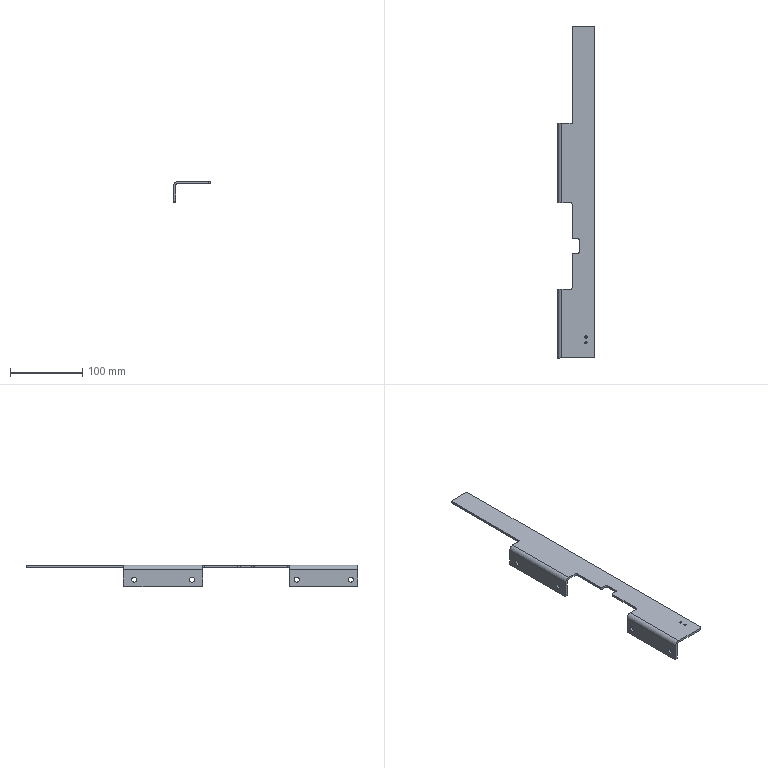Part | NX | features 5003_221_Bracket 2 | 1 solid | 43 faces | box 51 x 460 x 30 mm | volume 69398 mm3 | cylinder 21 | plane 20 | cone 2 | commonest cylinder face diameters 4 x11 7 x4 2.5 x2 6 x2 12 x2
STEP:
#1=CARTESIAN_POINT('',(224.525,-262.,-58.));
#2=VERTEX_POINT('',#1);
#3=CARTESIAN_POINT('',(224.525,-152.,-58.));
#4=VERTEX_POINT('',#3);
#5=CARTESIAN_POINT('',(224.525,-477.,-58.));
#6=DIRECTION('',(0.,1.,0.));
#7=VECTOR('',#6,1000.);
#8=LINE('',#5,#7);
#9=EDGE_CURVE('',#2,#4,#8,.T.);
#10=ORIENTED_EDGE('',*,*,#9,.T.);
#11=CARTESIAN_POINT('',(218.525,-152.,-64.));
#12=VERTEX_POINT('',#11);
#13=CARTESIAN_POINT('',(224.525,-152.,-64.));
#14=DIRECTION('',(0.,-1.,0.));
#15=DIRECTION('',(1.,0.,0.));
#16=AXIS2_PLACEMENT_3D('',#13,#14,#15);
#17=CIRCLE('',#16,6.);
#18=EDGE_CURVE('',#12,#4,#17,.F.);
#19=ORIENTED_EDGE('',*,*,#18,.F.);
#20=CARTESIAN_POINT('',(218.525,-262.,-64.));
#21=VERTEX_POINT('',#20);
#22=CARTESIAN_POINT('',(218.525,-477.,-64.));
#23=DIRECTION('',(0.,1.,0.));
#24=VECTOR('',#23,1000.);
#25=LINE('',#22,#24);
#26=EDGE_CURVE('',#21,#12,#25,.T.);
#27=ORIENTED_EDGE('',*,*,#26,.F.);
#28=CARTESIAN_POINT('',(224.525,-262.,-64.));
#29=DIRECTION('',(0.,1.,0.));
#30=DIRECTION('',(-1.,0.,0.));
#31=AXIS2_PLACEMENT_3D('',#28,#29,#30);
#32=CIRCLE('',#31,6.);
#33=EDGE_CURVE('',#2,#21,#32,.F.);
#34=ORIENTED_EDGE('',*,*,#33,.F.);
#35=EDGE_LOOP('',(#10,#19,#27,#34));
#36=FACE_BOUND('',#35,.T.);
#37=CARTESIAN_POINT('',(224.525,-477.,-64.));
#38=DIRECTION('',(0.,1.,0.));
#39=DIRECTION('',(-1.,0.,0.));
#40=AXIS2_PLACEMENT_3D('',#37,#38,#39);
#41=CYLINDRICAL_SURFACE('',#40,6.);
#42=ADVANCED_FACE('',(#36),#41,.T.);
#43=CARTESIAN_POINT('',(218.525,-167.,-74.5));
#44=VERTEX_POINT('',#43);
#45=CARTESIAN_POINT('',(218.525,-167.,-78.));
#46=DIRECTION('',(1.,0.,0.));
#47=DIRECTION('',(0.,0.,1.));
#48=AXIS2_PLACEMENT_3D('',#45,#46,#47);
#49=CIRCLE('',#48,3.5);
#50=EDGE_CURVE('',#44,#44,#49,.T.);
#51=ORIENTED_EDGE('',*,*,#50,.T.);
#52=EDGE_LOOP('',(#51));
#53=FACE_BOUND('',#52,.T.);
#54=CARTESIAN_POINT('',(218.525,-247.,-74.5));
#55=VERTEX_POINT('',#54);
#56=CARTESIAN_POINT('',(218.525,-247.,-78.));
#57=DIRECTION('',(1.,0.,0.));
#58=DIRECTION('',(0.,0.,1.));
#59=AXIS2_PLACEMENT_3D('',#56,#57,#58);
#60=CIRCLE('',#59,3.5);
#61=EDGE_CURVE('',#55,#55,#60,.T.);
#62=ORIENTED_EDGE('',*,*,#61,.T.);
#63=EDGE_LOOP('',(#62));
#64=FACE_BOUND('',#63,.T.);
#65=CARTESIAN_POINT('',(218.525,-152.,-86.));
#66=VERTEX_POINT('',#65);
#67=CARTESIAN_POINT('',(218.525,-152.,-57.999));
#68=DIRECTION('',(0.,0.,-1.));
#69=VECTOR('',#68,1000.);
#70=LINE('',#67,#69);
#71=EDGE_CURVE('',#12,#66,#70,.T.);
#72=ORIENTED_EDGE('',*,*,#71,.T.);
#73=CARTESIAN_POINT('',(218.525,-154.,-88.));
#74=VERTEX_POINT('',#73);
#75=CARTESIAN_POINT('',(218.525,-154.,-86.));
#76=DIRECTION('',(1.,0.,0.));
#77=DIRECTION('',(0.,0.,1.));
#78=AXIS2_PLACEMENT_3D('',#75,#76,#77);
#79=CIRCLE('',#78,2.);
#80=EDGE_CURVE('',#66,#74,#79,.F.);
#81=ORIENTED_EDGE('',*,*,#80,.T.);
#82=CARTESIAN_POINT('',(218.525,-260.,-88.));
#83=VERTEX_POINT('',#82);
#84=CARTESIAN_POINT('',(218.525,-477.,-88.));
#85=DIRECTION('',(0.,1.,0.));
#86=VECTOR('',#85,1000.);
#87=LINE('',#84,#86);
#88=EDGE_CURVE('',#83,#74,#87,.T.);
#89=ORIENTED_EDGE('',*,*,#88,.F.);
#90=CARTESIAN_POINT('',(218.525,-262.,-86.));
#91=VERTEX_POINT('',#90);
#92=CARTESIAN_POINT('',(218.525,-260.,-86.));
#93=DIRECTION('',(1.,0.,0.));
#94=DIRECTION('',(0.,0.,1.));
#95=AXIS2_PLACEMENT_3D('',#92,#93,#94);
#96=CIRCLE('',#95,2.);
#97=EDGE_CURVE('',#83,#91,#96,.F.);
#98=ORIENTED_EDGE('',*,*,#97,.T.);
#99=CARTESIAN_POINT('',(218.525,-262.,-57.999));
#100=DIRECTION('',(0.,0.,-1.));
#101=VECTOR('',#100,1000.);
#102=LINE('',#99,#101);
#103=EDGE_CURVE('',#21,#91,#102,.T.);
#104=ORIENTED_EDGE('',*,*,#103,.F.);
#105=ORIENTED_EDGE('',*,*,#26,.T.);
#106=EDGE_LOOP('',(#72,#81,#89,#98,#104,#105));
#107=FACE_BOUND('',#106,.T.);
#108=CARTESIAN_POINT('',(218.525,-477.,-64.));
#109=DIRECTION('',(1.,0.,0.));
#110=DIRECTION('',(0.,0.,1.));
#111=AXIS2_PLACEMENT_3D('',#108,#109,#110);
#112=PLANE('',#111);
#113=ADVANCED_FACE('',(#53,#64,#107),#112,.F.);
#114=ORIENTED_EDGE('',*,*,#88,.T.);
#115=CARTESIAN_POINT('',(221.525,-154.,-88.));
#116=VERTEX_POINT('',#115);
#117=CARTESIAN_POINT('',(218.525,-154.,-88.));
#118=DIRECTION('',(-1.,0.,0.));
#119=VECTOR('',#118,1000.);
#120=LINE('',#117,#119);
#121=EDGE_CURVE('',#74,#116,#120,.F.);
#122=ORIENTED_EDGE('',*,*,#121,.T.);
#123=CARTESIAN_POINT('',(221.525,-260.,-88.));
#124=VERTEX_POINT('',#123);
#125=CARTESIAN_POINT('',(221.525,-477.,-88.));
#126=DIRECTION('',(0.,1.,0.));
#127=VECTOR('',#126,1000.);
#128=LINE('',#125,#127);
#129=EDGE_CURVE('',#124,#116,#128,.T.);
#130=ORIENTED_EDGE('',*,*,#129,.F.);
#131=CARTESIAN_POINT('',(218.525,-260.,-88.));
#132=DIRECTION('',(1.,0.,0.));
#133=VECTOR('',#132,1000.);
#134=LINE('',#131,#133);
#135=EDGE_CURVE('',#124,#83,#134,.F.);
#136=ORIENTED_EDGE('',*,*,#135,.T.);
#137=EDGE_LOOP('',(#114,#122,#130,#136));
#138=FACE_BOUND('',#137,.T.);
#139=CARTESIAN_POINT('',(218.525,-477.,-88.));
#140=DIRECTION('',(0.,0.,1.));
#141=DIRECTION('',(0.,-1.,0.));
#142=AXIS2_PLACEMENT_3D('',#139,#140,#141);
#143=PLANE('',#142);
#144=ADVANCED_FACE('',(#138),#143,.F.);
#145=CARTESIAN_POINT('',(221.525,-167.,-74.5));
#146=VERTEX_POINT('',#145);
#147=CARTESIAN_POINT('',(221.525,-167.,-78.));
#148=DIRECTION('',(1.,0.,0.));
#149=DIRECTION('',(0.,0.,1.));
#150=AXIS2_PLACEMENT_3D('',#147,#148,#149);
#151=CIRCLE('',#150,3.5);
#152=EDGE_CURVE('',#146,#146,#151,.T.);
#153=ORIENTED_EDGE('',*,*,#152,.F.);
#154=EDGE_LOOP('',(#153));
#155=FACE_BOUND('',#154,.T.);
#156=CARTESIAN_POINT('',(221.525,-247.,-74.5));
#157=VERTEX_POINT('',#156);
#158=CARTESIAN_POINT('',(221.525,-247.,-78.));
#159=DIRECTION('',(1.,0.,0.));
#160=DIRECTION('',(0.,0.,1.));
#161=AXIS2_PLACEMENT_3D('',#158,#159,#160);
#162=CIRCLE('',#161,3.5);
#163=EDGE_CURVE('',#157,#157,#162,.T.);
#164=ORIENTED_EDGE('',*,*,#163,.F.);
#165=EDGE_LOOP('',(#164));
#166=FACE_BOUND('',#165,.T.);
#167=ORIENTED_EDGE('',*,*,#129,.T.);
#168=CARTESIAN_POINT('',(221.525,-152.,-86.));
#169=VERTEX_POINT('',#168);
#170=CARTESIAN_POINT('',(221.525,-154.,-86.));
#171=DIRECTION('',(-1.,0.,0.));
#172=DIRECTION('',(0.,0.,-1.));
#173=AXIS2_PLACEMENT_3D('',#170,#171,#172);
#174=CIRCLE('',#173,2.);
#175=EDGE_CURVE('',#116,#169,#174,.F.);
#176=ORIENTED_EDGE('',*,*,#175,.T.);
#177=CARTESIAN_POINT('',(221.525,-152.,-64.));
#178=VERTEX_POINT('',#177);
#179=CARTESIAN_POINT('',(221.525,-152.,-57.999));
#180=DIRECTION('',(0.,0.,-1.));
#181=VECTOR('',#180,1000.);
#182=LINE('',#179,#181);
#183=EDGE_CURVE('',#178,#169,#182,.T.);
#184=ORIENTED_EDGE('',*,*,#183,.F.);
#185=CARTESIAN_POINT('',(221.525,-262.,-64.));
#186=VERTEX_POINT('',#185);
#187=CARTESIAN_POINT('',(221.525,-477.,-64.));
#188=DIRECTION('',(0.,1.,0.));
#189=VECTOR('',#188,1000.);
#190=LINE('',#187,#189);
#191=EDGE_CURVE('',#186,#178,#190,.T.);
#192=ORIENTED_EDGE('',*,*,#191,.F.);
#193=CARTESIAN_POINT('',(221.525,-262.,-86.));
#194=VERTEX_POINT('',#193);
#195=CARTESIAN_POINT('',(221.525,-262.,-57.999));
#196=DIRECTION('',(0.,0.,1.));
#197=VECTOR('',#196,1000.);
#198=LINE('',#195,#197);
#199=EDGE_CURVE('',#194,#186,#198,.T.);
#200=ORIENTED_EDGE('',*,*,#199,.F.);
#201=CARTESIAN_POINT('',(221.525,-260.,-86.));
#202=DIRECTION('',(-1.,0.,0.));
#203=DIRECTION('',(0.,0.,-1.));
#204=AXIS2_PLACEMENT_3D('',#201,#202,#203);
#205=CIRCLE('',#204,2.);
#206=EDGE_CURVE('',#194,#124,#205,.F.);
#207=ORIENTED_EDGE('',*,*,#206,.T.);
#208=EDGE_LOOP('',(#167,#176,#184,#192,#200,#207));
#209=FACE_BOUND('',#208,.T.);
#210=CARTESIAN_POINT('',(221.525,-477.,-88.));
#211=DIRECTION('',(-1.,0.,0.));
#212=DIRECTION('',(0.,0.,-1.));
#213=AXIS2_PLACEMENT_3D('',#210,#211,#212);
#214=PLANE('',#213);
#215=ADVANCED_FACE('',(#155,#166,#209),#214,.F.);
#216=ORIENTED_EDGE('',*,*,#191,.T.);
#217=CARTESIAN_POINT('',(224.525,-152.,-61.));
#218=VERTEX_POINT('',#217);
#219=CARTESIAN_POINT('',(224.525,-152.,-64.));
#220=DIRECTION('',(0.,-1.,0.));
#221=DIRECTION('',(1.,0.,0.));
#222=AXIS2_PLACEMENT_3D('',#219,#220,#221);
#223=CIRCLE('',#222,3.);
#224=EDGE_CURVE('',#218,#178,#223,.T.);
#225=ORIENTED_EDGE('',*,*,#224,.F.);
#226=CARTESIAN_POINT('',(224.525,-262.,-61.));
#227=VERTEX_POINT('',#226);
#228=CARTESIAN_POINT('',(224.525,-477.,-61.));
#229=DIRECTION('',(0.,1.,0.));
#230=VECTOR('',#229,1000.);
#231=LINE('',#228,#230);
#232=EDGE_CURVE('',#227,#218,#231,.T.);
#233=ORIENTED_EDGE('',*,*,#232,.F.);
#234=CARTESIAN_POINT('',(224.525,-262.,-64.));
#235=DIRECTION('',(0.,1.,0.));
#236=DIRECTION('',(-1.,0.,0.));
#237=AXIS2_PLACEMENT_3D('',#234,#235,#236);
#238=CIRCLE('',#237,3.);
#239=EDGE_CURVE('',#186,#227,#238,.T.);
#240=ORIENTED_EDGE('',*,*,#239,.F.);
#241=EDGE_LOOP('',(#216,#225,#233,#240));
#242=FACE_BOUND('',#241,.T.);
#243=CARTESIAN_POINT('',(224.525,-477.,-64.));
#244=DIRECTION('',(0.,1.,0.));
#245=DIRECTION('',(-1.,0.,0.));
#246=AXIS2_PLACEMENT_3D('',#243,#244,#245);
#247=CYLINDRICAL_SURFACE('',#246,3.);
#248=ADVANCED_FACE('',(#242),#247,.F.);
#249=CARTESIAN_POINT('',(269.525,-475.,-61.));
#250=VERTEX_POINT('',#249);
#251=CARTESIAN_POINT('',(269.525,-19.,-61.));
#252=VERTEX_POINT('',#251);
#253=CARTESIAN_POINT('',(269.525,-477.,-61.));
#254=DIRECTION('',(0.,1.,0.));
#255=VECTOR('',#254,1000.);
#256=LINE('',#253,#255);
#257=EDGE_CURVE('',#250,#252,#256,.T.);
#258=ORIENTED_EDGE('',*,*,#257,.T.);
#259=CARTESIAN_POINT('',(269.525,-19.,-58.));
#260=VERTEX_POINT('',#259);
#261=CARTESIAN_POINT('',(269.525,-19.,-58.));
#262=DIRECTION('',(0.,0.,1.));
#263=VECTOR('',#262,1000.);
#264=LINE('',#261,#263);
#265=EDGE_CURVE('',#252,#260,#264,.T.);
#266=ORIENTED_EDGE('',*,*,#265,.T.);
#267=CARTESIAN_POINT('',(269.525,-475.,-58.));
#268=VERTEX_POINT('',#267);
#269=CARTESIAN_POINT('',(269.525,-477.,-58.));
#270=DIRECTION('',(0.,1.,0.));
#271=VECTOR('',#270,1000.);
#272=LINE('',#269,#271);
#273=EDGE_CURVE('',#268,#260,#272,.T.);
#274=ORIENTED_EDGE('',*,*,#273,.F.);
#275=CARTESIAN_POINT('',(269.525,-475.,-58.));
#276=DIRECTION('',(0.,0.,1.));
#277=VECTOR('',#276,1000.);
#278=LINE('',#275,#277);
#279=EDGE_CURVE('',#268,#250,#278,.F.);
#280=ORIENTED_EDGE('',*,*,#279,.T.);
#281=EDGE_LOOP('',(#258,#266,#274,#280));
#282=FACE_BOUND('',#281,.T.);
#283=CARTESIAN_POINT('',(269.525,-477.,-58.));
#284=DIRECTION('',(-1.,0.,0.));
#285=DIRECTION('',(0.,-1.,0.));
#286=AXIS2_PLACEMENT_3D('',#283,#284,#285);
#287=PLANE('',#286);
#288=ADVANCED_FACE('',(#282),#287,.F.);
#289=CARTESIAN_POINT('',(257.825,-457.565,-58.));
#290=VERTEX_POINT('',#289);
#291=CARTESIAN_POINT('',(257.825,-456.04,-58.));
#292=DIRECTION('',(0.,0.,1.));
#293=DIRECTION('',(0.,-1.,0.));
#294=AXIS2_PLACEMENT_3D('',#291,#292,#293);
#295=CIRCLE('',#294,1.525);
#296=EDGE_CURVE('',#290,#290,#295,.T.);
#297=ORIENTED_EDGE('',*,*,#296,.F.);
#298=EDGE_LOOP('',(#297));
#299=FACE_BOUND('',#298,.T.);
#300=CARTESIAN_POINT('',(257.825,-449.565,-58.));
#301=VERTEX_POINT('',#300);
#302=CARTESIAN_POINT('',(257.825,-448.04,-58.));
#303=DIRECTION('',(0.,0.,1.));
#304=DIRECTION('',(0.,-1.,0.));
#305=AXIS2_PLACEMENT_3D('',#302,#303,#304);
#306=CIRCLE('',#305,1.525);
#307=EDGE_CURVE('',#301,#301,#306,.T.);
#308=ORIENTED_EDGE('',*,*,#307,.F.);
#309=EDGE_LOOP('',(#308));
#310=FACE_BOUND('',#309,.T.);
#311=CARTESIAN_POINT('',(238.525,-310.,-58.));
#312=VERTEX_POINT('',#311);
#313=CARTESIAN_POINT('',(238.525,-264.,-58.));
#314=VERTEX_POINT('',#313);
#315=CARTESIAN_POINT('',(238.525,-312.,-58.));
#316=DIRECTION('',(0.,1.,0.));
#317=VECTOR('',#316,1000.);
#318=LINE('',#315,#317);
#319=EDGE_CURVE('',#312,#314,#318,.T.);
#320=ORIENTED_EDGE('',*,*,#319,.F.);
#321=CARTESIAN_POINT('',(240.525,-312.,-58.));
#322=VERTEX_POINT('',#321);
#323=CARTESIAN_POINT('',(240.525,-310.,-58.));
#324=DIRECTION('',(0.,0.,-1.));
#325=DIRECTION('',(0.,1.,0.));
#326=AXIS2_PLACEMENT_3D('',#323,#324,#325);
#327=CIRCLE('',#326,2.);
#328=EDGE_CURVE('',#312,#322,#327,.F.);
#329=ORIENTED_EDGE('',*,*,#328,.T.);
#330=CARTESIAN_POINT('',(246.525,-312.,-58.));
#331=VERTEX_POINT('',#330);
#332=CARTESIAN_POINT('',(248.525,-312.,-58.));
#333=DIRECTION('',(-1.,0.,0.));
#334=VECTOR('',#333,1000.);
#335=LINE('',#332,#334);
#336=EDGE_CURVE('',#331,#322,#335,.T.);
#337=ORIENTED_EDGE('',*,*,#336,.F.);
#338=CARTESIAN_POINT('',(248.525,-314.,-58.));
#339=VERTEX_POINT('',#338);
#340=CARTESIAN_POINT('',(246.525,-314.,-58.));
#341=DIRECTION('',(0.,0.,-1.));
#342=DIRECTION('',(0.,1.,0.));
#343=AXIS2_PLACEMENT_3D('',#340,#341,#342);
#344=CIRCLE('',#343,2.);
#345=EDGE_CURVE('',#331,#339,#344,.T.);
#346=ORIENTED_EDGE('',*,*,#345,.T.);
#347=CARTESIAN_POINT('',(248.525,-330.,-58.));
#348=VERTEX_POINT('',#347);
#349=CARTESIAN_POINT('',(248.525,-332.,-58.));
#350=DIRECTION('',(0.,1.,0.));
#351=VECTOR('',#350,1000.);
#352=LINE('',#349,#351);
#353=EDGE_CURVE('',#348,#339,#352,.T.);
#354=ORIENTED_EDGE('',*,*,#353,.F.);
#355=CARTESIAN_POINT('',(246.525,-332.,-58.));
#356=VERTEX_POINT('',#355);
#357=CARTESIAN_POINT('',(246.525,-330.,-58.));
#358=DIRECTION('',(0.,0.,-1.));
#359=DIRECTION('',(0.,1.,0.));
#360=AXIS2_PLACEMENT_3D('',#357,#358,#359);
#361=CIRCLE('',#360,2.);
#362=EDGE_CURVE('',#348,#356,#361,.T.);
#363=ORIENTED_EDGE('',*,*,#362,.T.);
#364=CARTESIAN_POINT('',(240.525,-332.,-58.));
#365=VERTEX_POINT('',#364);
#366=CARTESIAN_POINT('',(238.525,-332.,-58.));
#367=DIRECTION('',(1.,0.,0.));
#368=VECTOR('',#367,1000.);
#369=LINE('',#366,#368);
#370=EDGE_CURVE('',#365,#356,#369,.T.);
#371=ORIENTED_EDGE('',*,*,#370,.F.);
#372=CARTESIAN_POINT('',(238.525,-334.,-58.));
#373=VERTEX_POINT('',#372);
#374=CARTESIAN_POINT('',(240.525,-334.,-58.));
#375=DIRECTION('',(0.,0.,-1.));
#376=DIRECTION('',(0.,1.,0.));
#377=AXIS2_PLACEMENT_3D('',#374,#375,#376);
#378=CIRCLE('',#377,2.);
#379=EDGE_CURVE('',#365,#373,#378,.F.);
#380=ORIENTED_EDGE('',*,*,#379,.T.);
#381=CARTESIAN_POINT('',(238.525,-380.,-58.));
#382=VERTEX_POINT('',#381);
#383=CARTESIAN_POINT('',(238.525,-382.,-58.));
#384=DIRECTION('',(0.,1.,0.));
#385=VECTOR('',#384,1000.);
#386=LINE('',#383,#385);
#387=EDGE_CURVE('',#382,#373,#386,.T.);
#388=ORIENTED_EDGE('',*,*,#387,.F.);
#389=CARTESIAN_POINT('',(236.525,-382.,-58.));
#390=VERTEX_POINT('',#389);
#391=CARTESIAN_POINT('',(236.525,-380.,-58.));
#392=DIRECTION('',(0.,0.,-1.));
#393=DIRECTION('',(0.,1.,0.));
#394=AXIS2_PLACEMENT_3D('',#391,#392,#393);
#395=CIRCLE('',#394,2.);
#396=EDGE_CURVE('',#382,#390,#395,.T.);
#397=ORIENTED_EDGE('',*,*,#396,.T.);
#398=CARTESIAN_POINT('',(224.525,-382.,-58.));
#399=VERTEX_POINT('',#398);
#400=CARTESIAN_POINT('',(238.525,-382.,-58.));
#401=DIRECTION('',(1.,0.,0.));
#402=VECTOR('',#401,1000.);
#403=LINE('',#400,#402);
#404=EDGE_CURVE('',#399,#390,#403,.T.);
#405=ORIENTED_EDGE('',*,*,#404,.F.);
#406=CARTESIAN_POINT('',(224.525,-477.,-58.));
#407=VERTEX_POINT('',#406);
#408=CARTESIAN_POINT('',(224.525,-477.,-58.));
#409=DIRECTION('',(0.,1.,0.));
#410=VECTOR('',#409,1000.);
#411=LINE('',#408,#410);
#412=EDGE_CURVE('',#407,#399,#411,.T.);
#413=ORIENTED_EDGE('',*,*,#412,.F.);
#414=CARTESIAN_POINT('',(267.525,-477.,-58.));
#415=VERTEX_POINT('',#414);
#416=CARTESIAN_POINT('',(224.525,-477.,-58.));
#417=DIRECTION('',(-1.,0.,0.));
#418=VECTOR('',#417,1000.);
#419=LINE('',#416,#418);
#420=EDGE_CURVE('',#415,#407,#419,.T.);
#421=ORIENTED_EDGE('',*,*,#420,.F.);
#422=CARTESIAN_POINT('',(267.525,-475.,-58.));
#423=DIRECTION('',(0.,0.,-1.));
#424=DIRECTION('',(0.,1.,0.));
#425=AXIS2_PLACEMENT_3D('',#422,#423,#424);
#426=CIRCLE('',#425,2.);
#427=EDGE_CURVE('',#415,#268,#426,.F.);
#428=ORIENTED_EDGE('',*,*,#427,.T.);
#429=ORIENTED_EDGE('',*,*,#273,.T.);
#430=CARTESIAN_POINT('',(267.525,-17.,-58.));
#431=VERTEX_POINT('',#430);
#432=CARTESIAN_POINT('',(267.525,-19.,-58.));
#433=DIRECTION('',(0.,0.,-1.));
#434=DIRECTION('',(0.,1.,0.));
#435=AXIS2_PLACEMENT_3D('',#432,#433,#434);
#436=CIRCLE('',#435,2.);
#437=EDGE_CURVE('',#260,#431,#436,.F.);
#438=ORIENTED_EDGE('',*,*,#437,.T.);
#439=CARTESIAN_POINT('',(238.525,-17.,-58.));
#440=VERTEX_POINT('',#439);
#441=CARTESIAN_POINT('',(224.525,-17.,-58.));
#442=DIRECTION('',(-1.,0.,0.));
#443=VECTOR('',#442,1000.);
#444=LINE('',#441,#443);
#445=EDGE_CURVE('',#431,#440,#444,.T.);
#446=ORIENTED_EDGE('',*,*,#445,.T.);
#447=CARTESIAN_POINT('',(238.525,-152.,-58.));
#448=VERTEX_POINT('',#447);
#449=CARTESIAN_POINT('',(238.525,-152.,-58.));
#450=DIRECTION('',(0.,1.,0.));
#451=VECTOR('',#450,1000.);
#452=LINE('',#449,#451);
#453=EDGE_CURVE('',#448,#440,#452,.T.);
#454=ORIENTED_EDGE('',*,*,#453,.F.);
#455=CARTESIAN_POINT('',(218.525,-152.,-58.));
#456=DIRECTION('',(1.,0.,0.));
#457=VECTOR('',#456,1000.);
#458=LINE('',#455,#457);
#459=EDGE_CURVE('',#4,#448,#458,.T.);
#460=ORIENTED_EDGE('',*,*,#459,.F.);
#461=ORIENTED_EDGE('',*,*,#9,.F.);
#462=CARTESIAN_POINT('',(236.525,-262.,-58.));
#463=VERTEX_POINT('',#462);
#464=CARTESIAN_POINT('',(238.525,-262.,-58.));
#465=DIRECTION('',(-1.,0.,0.));
#466=VECTOR('',#465,1000.);
#467=LINE('',#464,#466);
#468=EDGE_CURVE('',#463,#2,#467,.T.);
#469=ORIENTED_EDGE('',*,*,#468,.F.);
#470=CARTESIAN_POINT('',(236.525,-264.,-58.));
#471=DIRECTION('',(0.,0.,-1.));
#472=DIRECTION('',(0.,1.,0.));
#473=AXIS2_PLACEMENT_3D('',#470,#471,#472);
#474=CIRCLE('',#473,2.);
#475=EDGE_CURVE('',#463,#314,#474,.T.);
#476=ORIENTED_EDGE('',*,*,#475,.T.);
#477=EDGE_LOOP('',(#320,#329,#337,#346,#354,#363,#371,#380,#388,#397,#405,#413,#421,#428,#429,#438,#446,#454,#460,#461,#469,#476));
#478=FACE_BOUND('',#477,.T.);
#479=CARTESIAN_POINT('',(224.525,-477.,-58.));
#480=DIRECTION('',(0.,0.,-1.));
#481=DIRECTION('',(0.,1.,0.));
#482=AXIS2_PLACEMENT_3D('',#479,#480,#481);
#483=PLANE('',#482);
#484=ADVANCED_FACE('',(#299,#310,#478),#483,.F.);
#485=ORIENTED_EDGE('',*,*,#412,.T.);
#486=CARTESIAN_POINT('',(218.525,-382.,-64.));
#487=VERTEX_POINT('',#486);
#488=CARTESIAN_POINT('',(224.525,-382.,-64.));
#489=DIRECTION('',(0.,-1.,0.));
#490=DIRECTION('',(1.,0.,0.));
#491=AXIS2_PLACEMENT_3D('',#488,#489,#490);
#492=CIRCLE('',#491,6.);
#493=EDGE_CURVE('',#487,#399,#492,.F.);
#494=ORIENTED_EDGE('',*,*,#493,.F.);
#495=CARTESIAN_POINT('',(218.525,-477.,-64.));
#496=VERTEX_POINT('',#495);
#497=CARTESIAN_POINT('',(218.525,-477.,-64.));
#498=DIRECTION('',(0.,1.,0.));
#499=VECTOR('',#498,1000.);
#500=LINE('',#497,#499);
#501=EDGE_CURVE('',#496,#487,#500,.T.);
#502=ORIENTED_EDGE('',*,*,#501,.F.);
#503=CARTESIAN_POINT('',(224.525,-477.,-64.));
#504=DIRECTION('',(0.,-1.,0.));
#505=DIRECTION('',(-1.,0.,0.));
#506=AXIS2_PLACEMENT_3D('',#503,#504,#505);
#507=CIRCLE('',#506,6.);
#508=EDGE_CURVE('',#407,#496,#507,.T.);
#509=ORIENTED_EDGE('',*,*,#508,.F.);
#510=EDGE_LOOP('',(#485,#494,#502,#509));
#511=FACE_BOUND('',#510,.T.);
#512=CARTESIAN_POINT('',(224.525,-477.,-64.));
#513=DIRECTION('',(0.,1.,0.));
#514=DIRECTION('',(-1.,0.,0.));
#515=AXIS2_PLACEMENT_3D('',#512,#513,#514);
#516=CYLINDRICAL_SURFACE('',#515,6.);
#517=ADVANCED_FACE('',(#511),#516,.T.);
#518=CARTESIAN_POINT('',(218.525,-467.,-74.5));
#519=VERTEX_POINT('',#518);
#520=CARTESIAN_POINT('',(218.525,-467.,-78.));
#521=DIRECTION('',(1.,0.,0.));
#522=DIRECTION('',(0.,0.,1.));
#523=AXIS2_PLACEMENT_3D('',#520,#521,#522);
#524=CIRCLE('',#523,3.5);
#525=EDGE_CURVE('',#519,#519,#524,.T.);
#526=ORIENTED_EDGE('',*,*,#525,.T.);
#527=EDGE_LOOP('',(#526));
#528=FACE_BOUND('',#527,.T.);
#529=CARTESIAN_POINT('',(218.525,-392.,-74.5));
#530=VERTEX_POINT('',#529);
#531=CARTESIAN_POINT('',(218.525,-392.,-78.));
#532=DIRECTION('',(1.,0.,0.));
#533=DIRECTION('',(0.,0.,1.));
#534=AXIS2_PLACEMENT_3D('',#531,#532,#533);
#535=CIRCLE('',#534,3.5);
#536=EDGE_CURVE('',#530,#530,#535,.T.);
#537=ORIENTED_EDGE('',*,*,#536,.T.);
#538=EDGE_LOOP('',(#537));
#539=FACE_BOUND('',#538,.T.);
#540=ORIENTED_EDGE('',*,*,#501,.T.);
#541=CARTESIAN_POINT('',(218.525,-382.,-88.));
#542=VERTEX_POINT('',#541);
#543=CARTESIAN_POINT('',(218.525,-382.,-57.999));
#544=DIRECTION('',(0.,0.,-1.));
#545=VECTOR('',#544,1000.);
#546=LINE('',#543,#545);
#547=EDGE_CURVE('',#487,#542,#546,.T.);
#548=ORIENTED_EDGE('',*,*,#547,.T.);
#549=CARTESIAN_POINT('',(218.525,-475.,-88.));
#550=VERTEX_POINT('',#549);
#551=CARTESIAN_POINT('',(218.525,-477.,-88.));
#552=DIRECTION('',(0.,1.,0.));
#553=VECTOR('',#552,1000.);
#554=LINE('',#551,#553);
#555=EDGE_CURVE('',#550,#542,#554,.T.);
#556=ORIENTED_EDGE('',*,*,#555,.F.);
#557=CARTESIAN_POINT('',(218.525,-477.,-86.));
#558=VERTEX_POINT('',#557);
#559=CARTESIAN_POINT('',(218.525,-475.,-86.));
#560=DIRECTION('',(1.,0.,0.));
#561=DIRECTION('',(0.,0.,1.));
#562=AXIS2_PLACEMENT_3D('',#559,#560,#561);
#563=CIRCLE('',#562,2.);
#564=EDGE_CURVE('',#550,#558,#563,.F.);
#565=ORIENTED_EDGE('',*,*,#564,.T.);
#566=CARTESIAN_POINT('',(218.525,-477.,-64.));
#567=DIRECTION('',(0.,0.,-1.));
#568=VECTOR('',#567,1000.);
#569=LINE('',#566,#568);
#570=EDGE_CURVE('',#496,#558,#569,.T.);
#571=ORIENTED_EDGE('',*,*,#570,.F.);
#572=EDGE_LOOP('',(#540,#548,#556,#565,#571));
#573=FACE_BOUND('',#572,.T.);
#574=CARTESIAN_POINT('',(218.525,-477.,-64.));
#575=DIRECTION('',(1.,0.,0.));
#576=DIRECTION('',(0.,0.,1.));
#577=AXIS2_PLACEMENT_3D('',#574,#575,#576);
#578=PLANE('',#577);
#579=ADVANCED_FACE('',(#528,#539,#573),#578,.F.);
#580=ORIENTED_EDGE('',*,*,#555,.T.);
#581=CARTESIAN_POINT('',(221.525,-382.,-88.));
#582=VERTEX_POINT('',#581);
#583=CARTESIAN_POINT('',(238.525,-382.,-88.));
#584=DIRECTION('',(-1.,0.,0.));
#585=VECTOR('',#584,1000.);
#586=LINE('',#583,#585);
#587=EDGE_CURVE('',#582,#542,#586,.T.);
#588=ORIENTED_EDGE('',*,*,#587,.F.);
#589=CARTESIAN_POINT('',(221.525,-475.,-88.));
#590=VERTEX_POINT('',#589);
#591=CARTESIAN_POINT('',(221.525,-477.,-88.));
#592=DIRECTION('',(0.,1.,0.));
#593=VECTOR('',#592,1000.);
#594=LINE('',#591,#593);
#595=EDGE_CURVE('',#590,#582,#594,.T.);
#596=ORIENTED_EDGE('',*,*,#595,.F.);
#597=CARTESIAN_POINT('',(218.525,-475.,-88.));
#598=DIRECTION('',(1.,0.,0.));
#599=VECTOR('',#598,1000.);
#600=LINE('',#597,#599);
#601=EDGE_CURVE('',#590,#550,#600,.F.);
#602=ORIENTED_EDGE('',*,*,#601,.T.);
#603=EDGE_LOOP('',(#580,#588,#596,#602));
#604=FACE_BOUND('',#603,.T.);
#605=CARTESIAN_POINT('',(218.525,-477.,-88.));
#606=DIRECTION('',(0.,0.,1.));
#607=DIRECTION('',(0.,-1.,0.));
#608=AXIS2_PLACEMENT_3D('',#605,#606,#607);
#609=PLANE('',#608);
#610=ADVANCED_FACE('',(#604),#609,.F.);
#611=CARTESIAN_POINT('',(221.525,-467.,-74.5));
#612=VERTEX_POINT('',#611);
#613=CARTESIAN_POINT('',(221.525,-467.,-78.));
#614=DIRECTION('',(1.,0.,0.));
#615=DIRECTION('',(0.,0.,1.));
#616=AXIS2_PLACEMENT_3D('',#613,#614,#615);
#617=CIRCLE('',#616,3.5);
#618=EDGE_CURVE('',#612,#612,#617,.T.);
#619=ORIENTED_EDGE('',*,*,#618,.F.);
#620=EDGE_LOOP('',(#619));
#621=FACE_BOUND('',#620,.T.);
#622=CARTESIAN_POINT('',(221.525,-392.,-74.5));
#623=VERTEX_POINT('',#622);
#624=CARTESIAN_POINT('',(221.525,-392.,-78.));
#625=DIRECTION('',(1.,0.,0.));
#626=DIRECTION('',(0.,0.,1.));
#627=AXIS2_PLACEMENT_3D('',#624,#625,#626);
#628=CIRCLE('',#627,3.5);
#629=EDGE_CURVE('',#623,#623,#628,.T.);
#630=ORIENTED_EDGE('',*,*,#629,.F.);
#631=EDGE_LOOP('',(#630));
#632=FACE_BOUND('',#631,.T.);
#633=ORIENTED_EDGE('',*,*,#595,.T.);
#634=CARTESIAN_POINT('',(221.525,-382.,-64.));
#635=VERTEX_POINT('',#634);
#636=CARTESIAN_POINT('',(221.525,-382.,-57.999));
#637=DIRECTION('',(0.,0.,-1.));
#638=VECTOR('',#637,1000.);
#639=LINE('',#636,#638);
#640=EDGE_CURVE('',#635,#582,#639,.T.);
#641=ORIENTED_EDGE('',*,*,#640,.F.);
#642=CARTESIAN_POINT('',(221.525,-477.,-64.));
#643=VERTEX_POINT('',#642);
#644=CARTESIAN_POINT('',(221.525,-477.,-64.));
#645=DIRECTION('',(0.,1.,0.));
#646=VECTOR('',#645,1000.);
#647=LINE('',#644,#646);
#648=EDGE_CURVE('',#643,#635,#647,.T.);
#649=ORIENTED_EDGE('',*,*,#648,.F.);
#650=CARTESIAN_POINT('',(221.525,-477.,-86.));
#651=VERTEX_POINT('',#650);
#652=CARTESIAN_POINT('',(221.525,-477.,-88.));
#653=DIRECTION('',(0.,0.,1.));
#654=VECTOR('',#653,1000.);
#655=LINE('',#652,#654);
#656=EDGE_CURVE('',#651,#643,#655,.T.);
#657=ORIENTED_EDGE('',*,*,#656,.F.);
#658=CARTESIAN_POINT('',(221.525,-475.,-86.));
#659=DIRECTION('',(-1.,0.,0.));
#660=DIRECTION('',(0.,0.,-1.));
#661=AXIS2_PLACEMENT_3D('',#658,#659,#660);
#662=CIRCLE('',#661,2.);
#663=EDGE_CURVE('',#651,#590,#662,.F.);
#664=ORIENTED_EDGE('',*,*,#663,.T.);
#665=EDGE_LOOP('',(#633,#641,#649,#657,#664));
#666=FACE_BOUND('',#665,.T.);
#667=CARTESIAN_POINT('',(221.525,-477.,-88.));
#668=DIRECTION('',(-1.,0.,0.));
#669=DIRECTION('',(0.,0.,-1.));
#670=AXIS2_PLACEMENT_3D('',#667,#668,#669);
#671=PLANE('',#670);
#672=ADVANCED_FACE('',(#621,#632,#666),#671,.F.);
#673=ORIENTED_EDGE('',*,*,#648,.T.);
#674=CARTESIAN_POINT('',(224.525,-382.,-61.));
#675=VERTEX_POINT('',#674);
#676=CARTESIAN_POINT('',(224.525,-382.,-64.));
#677=DIRECTION('',(0.,-1.,0.));
#678=DIRECTION('',(1.,0.,0.));
#679=AXIS2_PLACEMENT_3D('',#676,#677,#678);
#680=CIRCLE('',#679,3.);
#681=EDGE_CURVE('',#675,#635,#680,.T.);
#682=ORIENTED_EDGE('',*,*,#681,.F.);
#683=CARTESIAN_POINT('',(224.525,-477.,-61.));
#684=VERTEX_POINT('',#683);
#685=CARTESIAN_POINT('',(224.525,-477.,-61.));
#686=DIRECTION('',(0.,1.,0.));
#687=VECTOR('',#686,1000.);
#688=LINE('',#685,#687);
#689=EDGE_CURVE('',#684,#675,#688,.T.);
#690=ORIENTED_EDGE('',*,*,#689,.F.);
#691=CARTESIAN_POINT('',(224.525,-477.,-64.));
#692=DIRECTION('',(0.,1.,0.));
#693=DIRECTION('',(-1.,0.,0.));
#694=AXIS2_PLACEMENT_3D('',#691,#692,#693);
#695=CIRCLE('',#694,3.);
#696=EDGE_CURVE('',#643,#684,#695,.T.);
#697=ORIENTED_EDGE('',*,*,#696,.F.);
#698=EDGE_LOOP('',(#673,#682,#690,#697));
#699=FACE_BOUND('',#698,.T.);
#700=CARTESIAN_POINT('',(224.525,-477.,-64.));
#701=DIRECTION('',(0.,1.,0.));
#702=DIRECTION('',(-1.,0.,0.));
#703=AXIS2_PLACEMENT_3D('',#700,#701,#702);
#704=CYLINDRICAL_SURFACE('',#703,3.);
#705=ADVANCED_FACE('',(#699),#704,.F.);
#706=CARTESIAN_POINT('',(257.825,-457.29,-61.));
#707=VERTEX_POINT('',#706);
#708=CARTESIAN_POINT('',(257.825,-456.04,-61.));
#709=DIRECTION('',(0.,0.,1.));
#710=DIRECTION('',(0.,-1.,0.));
#711=AXIS2_PLACEMENT_3D('',#708,#709,#710);
#712=CIRCLE('',#711,1.25);
#713=EDGE_CURVE('',#707,#707,#712,.T.);
#714=ORIENTED_EDGE('',*,*,#713,.T.);
#715=EDGE_LOOP('',(#714));
#716=FACE_BOUND('',#715,.T.);
#717=CARTESIAN_POINT('',(257.825,-449.29,-61.));
#718=VERTEX_POINT('',#717);
#719=CARTESIAN_POINT('',(257.825,-448.04,-61.));
#720=DIRECTION('',(0.,0.,1.));
#721=DIRECTION('',(0.,-1.,0.));
#722=AXIS2_PLACEMENT_3D('',#719,#720,#721);
#723=CIRCLE('',#722,1.25);
#724=EDGE_CURVE('',#718,#718,#723,.T.);
#725=ORIENTED_EDGE('',*,*,#724,.T.);
#726=EDGE_LOOP('',(#725));
#727=FACE_BOUND('',#726,.T.);
#728=CARTESIAN_POINT('',(240.525,-312.,-61.));
#729=VERTEX_POINT('',#728);
#730=CARTESIAN_POINT('',(246.525,-312.,-61.));
#731=VERTEX_POINT('',#730);
#732=CARTESIAN_POINT('',(248.525,-312.,-61.));
#733=DIRECTION('',(1.,0.,0.));
#734=VECTOR('',#733,1000.);
#735=LINE('',#732,#734);
#736=EDGE_CURVE('',#729,#731,#735,.T.);
#737=ORIENTED_EDGE('',*,*,#736,.F.);
#738=CARTESIAN_POINT('',(238.525,-310.,-61.));
#739=VERTEX_POINT('',#738);
#740=CARTESIAN_POINT('',(240.525,-310.,-61.));
#741=DIRECTION('',(0.,0.,1.));
#742=DIRECTION('',(0.,-1.,0.));
#743=AXIS2_PLACEMENT_3D('',#740,#741,#742);
#744=CIRCLE('',#743,2.);
#745=EDGE_CURVE('',#729,#739,#744,.F.);
#746=ORIENTED_EDGE('',*,*,#745,.T.);
#747=CARTESIAN_POINT('',(238.525,-264.,-61.));
#748=VERTEX_POINT('',#747);
#749=CARTESIAN_POINT('',(238.525,-312.,-61.));
#750=DIRECTION('',(0.,-1.,0.));
#751=VECTOR('',#750,1000.);
#752=LINE('',#749,#751);
#753=EDGE_CURVE('',#748,#739,#752,.T.);
#754=ORIENTED_EDGE('',*,*,#753,.F.);
#755=CARTESIAN_POINT('',(236.525,-262.,-61.));
#756=VERTEX_POINT('',#755);
#757=CARTESIAN_POINT('',(236.525,-264.,-61.));
#758=DIRECTION('',(0.,0.,1.));
#759=DIRECTION('',(0.,-1.,0.));
#760=AXIS2_PLACEMENT_3D('',#757,#758,#759);
#761=CIRCLE('',#760,2.);
#762=EDGE_CURVE('',#748,#756,#761,.T.);
#763=ORIENTED_EDGE('',*,*,#762,.T.);
#764=CARTESIAN_POINT('',(238.525,-262.,-61.));
#765=DIRECTION('',(1.,0.,0.));
#766=VECTOR('',#765,1000.);
#767=LINE('',#764,#766);
#768=EDGE_CURVE('',#227,#756,#767,.T.);
#769=ORIENTED_EDGE('',*,*,#768,.F.);
#770=ORIENTED_EDGE('',*,*,#232,.T.);
#771=CARTESIAN_POINT('',(238.525,-152.,-61.));
#772=VERTEX_POINT('',#771);
#773=CARTESIAN_POINT('',(218.525,-152.,-61.));
#774=DIRECTION('',(-1.,0.,0.));
#775=VECTOR('',#774,1000.);
#776=LINE('',#773,#775);
#777=EDGE_CURVE('',#772,#218,#776,.T.);
#778=ORIENTED_EDGE('',*,*,#777,.F.);
#779=CARTESIAN_POINT('',(238.525,-17.,-61.));
#780=VERTEX_POINT('',#779);
#781=CARTESIAN_POINT('',(238.525,-152.,-61.));
#782=DIRECTION('',(0.,-1.,0.));
#783=VECTOR('',#782,1000.);
#784=LINE('',#781,#783);
#785=EDGE_CURVE('',#780,#772,#784,.T.);
#786=ORIENTED_EDGE('',*,*,#785,.F.);
#787=CARTESIAN_POINT('',(267.525,-17.,-61.));
#788=VERTEX_POINT('',#787);
#789=CARTESIAN_POINT('',(224.525,-17.,-61.));
#790=DIRECTION('',(1.,0.,0.));
#791=VECTOR('',#790,1000.);
#792=LINE('',#789,#791);
#793=EDGE_CURVE('',#780,#788,#792,.T.);
#794=ORIENTED_EDGE('',*,*,#793,.T.);
#795=CARTESIAN_POINT('',(267.525,-19.,-61.));
#796=DIRECTION('',(0.,0.,1.));
#797=DIRECTION('',(0.,-1.,0.));
#798=AXIS2_PLACEMENT_3D('',#795,#796,#797);
#799=CIRCLE('',#798,2.);
#800=EDGE_CURVE('',#788,#252,#799,.F.);
#801=ORIENTED_EDGE('',*,*,#800,.T.);
#802=ORIENTED_EDGE('',*,*,#257,.F.);
#803=CARTESIAN_POINT('',(267.525,-477.,-61.));
#804=VERTEX_POINT('',#803);
#805=CARTESIAN_POINT('',(267.525,-475.,-61.));
#806=DIRECTION('',(0.,0.,1.));
#807=DIRECTION('',(0.,-1.,0.));
#808=AXIS2_PLACEMENT_3D('',#805,#806,#807);
#809=CIRCLE('',#808,2.);
#810=EDGE_CURVE('',#250,#804,#809,.F.);
#811=ORIENTED_EDGE('',*,*,#810,.T.);
#812=CARTESIAN_POINT('',(224.525,-477.,-61.));
#813=DIRECTION('',(1.,0.,0.));
#814=VECTOR('',#813,1000.);
#815=LINE('',#812,#814);
#816=EDGE_CURVE('',#684,#804,#815,.T.);
#817=ORIENTED_EDGE('',*,*,#816,.F.);
#818=ORIENTED_EDGE('',*,*,#689,.T.);
#819=CARTESIAN_POINT('',(236.525,-382.,-61.));
#820=VERTEX_POINT('',#819);
#821=CARTESIAN_POINT('',(238.525,-382.,-61.));
#822=DIRECTION('',(-1.,0.,0.));
#823=VECTOR('',#822,1000.);
#824=LINE('',#821,#823);
#825=EDGE_CURVE('',#820,#675,#824,.T.);
#826=ORIENTED_EDGE('',*,*,#825,.F.);
#827=CARTESIAN_POINT('',(238.525,-380.,-61.));
#828=VERTEX_POINT('',#827);
#829=CARTESIAN_POINT('',(236.525,-380.,-61.));
#830=DIRECTION('',(0.,0.,1.));
#831=DIRECTION('',(0.,-1.,0.));
#832=AXIS2_PLACEMENT_3D('',#829,#830,#831);
#833=CIRCLE('',#832,2.);
#834=EDGE_CURVE('',#820,#828,#833,.T.);
#835=ORIENTED_EDGE('',*,*,#834,.T.);
#836=CARTESIAN_POINT('',(238.525,-334.,-61.));
#837=VERTEX_POINT('',#836);
#838=CARTESIAN_POINT('',(238.525,-382.,-61.));
#839=DIRECTION('',(0.,-1.,0.));
#840=VECTOR('',#839,1000.);
#841=LINE('',#838,#840);
#842=EDGE_CURVE('',#837,#828,#841,.T.);
#843=ORIENTED_EDGE('',*,*,#842,.F.);
#844=CARTESIAN_POINT('',(240.525,-332.,-61.));
#845=VERTEX_POINT('',#844);
#846=CARTESIAN_POINT('',(240.525,-334.,-61.));
#847=DIRECTION('',(0.,0.,1.));
#848=DIRECTION('',(0.,-1.,0.));
#849=AXIS2_PLACEMENT_3D('',#846,#847,#848);
#850=CIRCLE('',#849,2.);
#851=EDGE_CURVE('',#837,#845,#850,.F.);
#852=ORIENTED_EDGE('',*,*,#851,.T.);
#853=CARTESIAN_POINT('',(246.525,-332.,-61.));
#854=VERTEX_POINT('',#853);
#855=CARTESIAN_POINT('',(238.525,-332.,-61.));
#856=DIRECTION('',(-1.,0.,0.));
#857=VECTOR('',#856,1000.);
#858=LINE('',#855,#857);
#859=EDGE_CURVE('',#854,#845,#858,.T.);
#860=ORIENTED_EDGE('',*,*,#859,.F.);
#861=CARTESIAN_POINT('',(248.525,-330.,-61.));
#862=VERTEX_POINT('',#861);
#863=CARTESIAN_POINT('',(246.525,-330.,-61.));
#864=DIRECTION('',(0.,0.,1.));
#865=DIRECTION('',(0.,-1.,0.));
#866=AXIS2_PLACEMENT_3D('',#863,#864,#865);
#867=CIRCLE('',#866,2.);
#868=EDGE_CURVE('',#854,#862,#867,.T.);
#869=ORIENTED_EDGE('',*,*,#868,.T.);
#870=CARTESIAN_POINT('',(248.525,-314.,-61.));
#871=VERTEX_POINT('',#870);
#872=CARTESIAN_POINT('',(248.525,-332.,-61.));
#873=DIRECTION('',(0.,-1.,0.));
#874=VECTOR('',#873,1000.);
#875=LINE('',#872,#874);
#876=EDGE_CURVE('',#871,#862,#875,.T.);
#877=ORIENTED_EDGE('',*,*,#876,.F.);
#878=CARTESIAN_POINT('',(246.525,-314.,-61.));
#879=DIRECTION('',(0.,0.,1.));
#880=DIRECTION('',(0.,-1.,0.));
#881=AXIS2_PLACEMENT_3D('',#878,#879,#880);
#882=CIRCLE('',#881,2.);
#883=EDGE_CURVE('',#871,#731,#882,.T.);
#884=ORIENTED_EDGE('',*,*,#883,.T.);
#885=EDGE_LOOP('',(#737,#746,#754,#763,#769,#770,#778,#786,#794,#801,#802,#811,#817,#818,#826,#835,#843,#852,#860,#869,#877,#884));
#886=FACE_BOUND('',#885,.T.);
#887=CARTESIAN_POINT('',(224.525,-477.,-61.));
#888=DIRECTION('',(0.,0.,1.));
#889=DIRECTION('',(0.,-1.,0.));
#890=AXIS2_PLACEMENT_3D('',#887,#888,#889);
#891=PLANE('',#890);
#892=ADVANCED_FACE('',(#716,#727,#886),#891,.F.);
#893=ORIENTED_EDGE('',*,*,#570,.T.);
#894=CARTESIAN_POINT('',(224.525,-477.,-86.));
#895=DIRECTION('',(1.,0.,0.));
#896=VECTOR('',#895,1000.);
#897=LINE('',#894,#896);
#898=EDGE_CURVE('',#558,#651,#897,.T.);
#899=ORIENTED_EDGE('',*,*,#898,.T.);
#900=ORIENTED_EDGE('',*,*,#656,.T.);
#901=ORIENTED_EDGE('',*,*,#696,.T.);
#902=ORIENTED_EDGE('',*,*,#816,.T.);
#903=CARTESIAN_POINT('',(267.525,-477.,-64.));
#904=DIRECTION('',(0.,0.,1.));
#905=VECTOR('',#904,1000.);
#906=LINE('',#903,#905);
#907=EDGE_CURVE('',#804,#415,#906,.T.);
#908=ORIENTED_EDGE('',*,*,#907,.T.);
#909=ORIENTED_EDGE('',*,*,#420,.T.);
#910=ORIENTED_EDGE('',*,*,#508,.T.);
#911=EDGE_LOOP('',(#893,#899,#900,#901,#902,#908,#909,#910));
#912=FACE_BOUND('',#911,.T.);
#913=CARTESIAN_POINT('',(224.525,-477.,-64.));
#914=DIRECTION('',(0.,1.,0.));
#915=DIRECTION('',(-1.,0.,0.));
#916=AXIS2_PLACEMENT_3D('',#913,#914,#915);
#917=PLANE('',#916);
#918=ADVANCED_FACE('',(#912),#917,.F.);
#919=CARTESIAN_POINT('',(238.525,-17.,-57.999));
#920=DIRECTION('',(0.,0.,-1.));
#921=VECTOR('',#920,1000.);
#922=LINE('',#919,#921);
#923=EDGE_CURVE('',#440,#780,#922,.T.);
#924=ORIENTED_EDGE('',*,*,#923,.F.);
#925=ORIENTED_EDGE('',*,*,#445,.F.);
#926=CARTESIAN_POINT('',(267.525,-17.,-61.));
#927=DIRECTION('',(0.,0.,1.));
#928=VECTOR('',#927,1000.);
#929=LINE('',#926,#928);
#930=EDGE_CURVE('',#431,#788,#929,.F.);
#931=ORIENTED_EDGE('',*,*,#930,.T.);
#932=ORIENTED_EDGE('',*,*,#793,.F.);
#933=EDGE_LOOP('',(#924,#925,#931,#932));
#934=FACE_BOUND('',#933,.T.);
#935=CARTESIAN_POINT('',(224.525,-17.,-64.));
#936=DIRECTION('',(0.,1.,0.));
#937=DIRECTION('',(-1.,0.,0.));
#938=AXIS2_PLACEMENT_3D('',#935,#936,#937);
#939=PLANE('',#938);
#940=ADVANCED_FACE('',(#934),#939,.T.);
#941=ORIENTED_EDGE('',*,*,#50,.F.);
#942=EDGE_LOOP('',(#941));
#943=FACE_BOUND('',#942,.T.);
#944=ORIENTED_EDGE('',*,*,#152,.T.);
#945=EDGE_LOOP('',(#944));
#946=FACE_BOUND('',#945,.T.);
#947=CARTESIAN_POINT('',(218.525,-167.,-78.));
#948=DIRECTION('',(1.,0.,0.));
#949=DIRECTION('',(0.,0.,1.));
#950=AXIS2_PLACEMENT_3D('',#947,#948,#949);
#951=CYLINDRICAL_SURFACE('',#950,3.5);
#952=ADVANCED_FACE('',(#943,#946),#951,.F.);
#953=ORIENTED_EDGE('',*,*,#61,.F.);
#954=EDGE_LOOP('',(#953));
#955=FACE_BOUND('',#954,.T.);
#956=ORIENTED_EDGE('',*,*,#163,.T.);
#957=EDGE_LOOP('',(#956));
#958=FACE_BOUND('',#957,.T.);
#959=CARTESIAN_POINT('',(218.525,-247.,-78.));
#960=DIRECTION('',(1.,0.,0.));
#961=DIRECTION('',(0.,0.,1.));
#962=AXIS2_PLACEMENT_3D('',#959,#960,#961);
#963=CYLINDRICAL_SURFACE('',#962,3.5);
#964=ADVANCED_FACE('',(#955,#958),#963,.F.);
#965=ORIENTED_EDGE('',*,*,#536,.F.);
#966=EDGE_LOOP('',(#965));
#967=FACE_BOUND('',#966,.T.);
#968=ORIENTED_EDGE('',*,*,#629,.T.);
#969=EDGE_LOOP('',(#968));
#970=FACE_BOUND('',#969,.T.);
#971=CARTESIAN_POINT('',(218.525,-392.,-78.));
#972=DIRECTION('',(1.,0.,0.));
#973=DIRECTION('',(0.,0.,1.));
#974=AXIS2_PLACEMENT_3D('',#971,#972,#973);
#975=CYLINDRICAL_SURFACE('',#974,3.5);
#976=ADVANCED_FACE('',(#967,#970),#975,.F.);
#977=ORIENTED_EDGE('',*,*,#525,.F.);
#978=EDGE_LOOP('',(#977));
#979=FACE_BOUND('',#978,.T.);
#980=ORIENTED_EDGE('',*,*,#618,.T.);
#981=EDGE_LOOP('',(#980));
#982=FACE_BOUND('',#981,.T.);
#983=CARTESIAN_POINT('',(218.525,-467.,-78.));
#984=DIRECTION('',(1.,0.,0.));
#985=DIRECTION('',(0.,0.,1.));
#986=AXIS2_PLACEMENT_3D('',#983,#984,#985);
#987=CYLINDRICAL_SURFACE('',#986,3.5);
#988=ADVANCED_FACE('',(#979,#982),#987,.F.);
#989=CARTESIAN_POINT('',(257.825,-449.29,-58.275));
#990=VERTEX_POINT('',#989);
#991=CARTESIAN_POINT('',(257.825,-448.04,-58.275));
#992=DIRECTION('',(0.,0.,1.));
#993=DIRECTION('',(0.,-1.,0.));
#994=AXIS2_PLACEMENT_3D('',#991,#992,#993);
#995=CIRCLE('',#994,1.25);
#996=EDGE_CURVE('',#990,#990,#995,.T.);
#997=ORIENTED_EDGE('',*,*,#996,.T.);
#998=EDGE_LOOP('',(#997));
#999=FACE_BOUND('',#998,.T.);
#1000=ORIENTED_EDGE('',*,*,#724,.F.);
#1001=EDGE_LOOP('',(#1000));
#1002=FACE_BOUND('',#1001,.T.);
#1003=CARTESIAN_POINT('',(257.825,-448.04,-58.));
#1004=DIRECTION('',(0.,0.,1.));
#1005=DIRECTION('',(0.,-1.,0.));
#1006=AXIS2_PLACEMENT_3D('',#1003,#1004,#1005);
#1007=CYLINDRICAL_SURFACE('',#1006,1.25);
#1008=ADVANCED_FACE('',(#999,#1002),#1007,.F.);
#1009=ORIENTED_EDGE('',*,*,#996,.F.);
#1010=EDGE_LOOP('',(#1009));
#1011=FACE_BOUND('',#1010,.T.);
#1012=ORIENTED_EDGE('',*,*,#307,.T.);
#1013=EDGE_LOOP('',(#1012));
#1014=FACE_BOUND('',#1013,.T.);
#1015=CARTESIAN_POINT('',(257.825,-448.04,-58.));
#1016=DIRECTION('',(0.,0.,1.));
#1017=DIRECTION('',(0.,-1.,0.));
#1018=AXIS2_PLACEMENT_3D('',#1015,#1016,#1017);
#1019=CONICAL_SURFACE('',#1018,1.525,0.7854);
#1020=ADVANCED_FACE('',(#1011,#1014),#1019,.F.);
#1021=CARTESIAN_POINT('',(257.825,-457.29,-58.275));
#1022=VERTEX_POINT('',#1021);
#1023=CARTESIAN_POINT('',(257.825,-456.04,-58.275));
#1024=DIRECTION('',(0.,0.,1.));
#1025=DIRECTION('',(0.,-1.,0.));
#1026=AXIS2_PLACEMENT_3D('',#1023,#1024,#1025);
#1027=CIRCLE('',#1026,1.25);
#1028=EDGE_CURVE('',#1022,#1022,#1027,.T.);
#1029=ORIENTED_EDGE('',*,*,#1028,.T.);
#1030=EDGE_LOOP('',(#1029));
#1031=FACE_BOUND('',#1030,.T.);
#1032=ORIENTED_EDGE('',*,*,#713,.F.);
#1033=EDGE_LOOP('',(#1032));
#1034=FACE_BOUND('',#1033,.T.);
#1035=CARTESIAN_POINT('',(257.825,-456.04,-58.));
#1036=DIRECTION('',(0.,0.,1.));
#1037=DIRECTION('',(0.,-1.,0.));
#1038=AXIS2_PLACEMENT_3D('',#1035,#1036,#1037);
#1039=CYLINDRICAL_SURFACE('',#1038,1.25);
#1040=ADVANCED_FACE('',(#1031,#1034),#1039,.F.);
#1041=ORIENTED_EDGE('',*,*,#1028,.F.);
#1042=EDGE_LOOP('',(#1041));
#1043=FACE_BOUND('',#1042,.T.);
#1044=ORIENTED_EDGE('',*,*,#296,.T.);
#1045=EDGE_LOOP('',(#1044));
#1046=FACE_BOUND('',#1045,.T.);
#1047=CARTESIAN_POINT('',(257.825,-456.04,-58.));
#1048=DIRECTION('',(0.,0.,1.));
#1049=DIRECTION('',(0.,-1.,0.));
#1050=AXIS2_PLACEMENT_3D('',#1047,#1048,#1049);
#1051=CONICAL_SURFACE('',#1050,1.525,0.7854);
#1052=ADVANCED_FACE('',(#1043,#1046),#1051,.F.);
#1053=ORIENTED_EDGE('',*,*,#800,.F.);
#1054=ORIENTED_EDGE('',*,*,#930,.F.);
#1055=ORIENTED_EDGE('',*,*,#437,.F.);
#1056=ORIENTED_EDGE('',*,*,#265,.F.);
#1057=EDGE_LOOP('',(#1053,#1054,#1055,#1056));
#1058=FACE_BOUND('',#1057,.T.);
#1059=CARTESIAN_POINT('',(267.525,-19.,-58.));
#1060=DIRECTION('',(0.,0.,-1.));
#1061=DIRECTION('',(0.,1.,0.));
#1062=AXIS2_PLACEMENT_3D('',#1059,#1060,#1061);
#1063=CYLINDRICAL_SURFACE('',#1062,2.);
#1064=ADVANCED_FACE('',(#1058),#1063,.T.);
#1065=ORIENTED_EDGE('',*,*,#564,.F.);
#1066=ORIENTED_EDGE('',*,*,#601,.F.);
#1067=ORIENTED_EDGE('',*,*,#663,.F.);
#1068=ORIENTED_EDGE('',*,*,#898,.F.);
#1069=EDGE_LOOP('',(#1065,#1066,#1067,#1068));
#1070=FACE_BOUND('',#1069,.T.);
#1071=CARTESIAN_POINT('',(224.525,-475.,-86.));
#1072=DIRECTION('',(1.,0.,0.));
#1073=DIRECTION('',(0.,1.,0.));
#1074=AXIS2_PLACEMENT_3D('',#1071,#1072,#1073);
#1075=CYLINDRICAL_SURFACE('',#1074,2.);
#1076=ADVANCED_FACE('',(#1070),#1075,.T.);
#1077=ORIENTED_EDGE('',*,*,#810,.F.);
#1078=ORIENTED_EDGE('',*,*,#279,.F.);
#1079=ORIENTED_EDGE('',*,*,#427,.F.);
#1080=ORIENTED_EDGE('',*,*,#907,.F.);
#1081=EDGE_LOOP('',(#1077,#1078,#1079,#1080));
#1082=FACE_BOUND('',#1081,.T.);
#1083=CARTESIAN_POINT('',(267.525,-475.,-64.));
#1084=DIRECTION('',(0.,0.,1.));
#1085=DIRECTION('',(0.,-1.,0.));
#1086=AXIS2_PLACEMENT_3D('',#1083,#1084,#1085);
#1087=CYLINDRICAL_SURFACE('',#1086,2.);
#1088=ADVANCED_FACE('',(#1082),#1087,.T.);
#1089=ORIENTED_EDGE('',*,*,#387,.T.);
#1090=CARTESIAN_POINT('',(238.525,-334.,-57.999));
#1091=DIRECTION('',(0.,0.,-1.));
#1092=VECTOR('',#1091,1000.);
#1093=LINE('',#1090,#1092);
#1094=EDGE_CURVE('',#373,#837,#1093,.T.);
#1095=ORIENTED_EDGE('',*,*,#1094,.T.);
#1096=ORIENTED_EDGE('',*,*,#842,.T.);
#1097=CARTESIAN_POINT('',(238.525,-380.,-58.));
#1098=DIRECTION('',(0.,0.,-1.));
#1099=VECTOR('',#1098,1000.);
#1100=LINE('',#1097,#1099);
#1101=EDGE_CURVE('',#828,#382,#1100,.F.);
#1102=ORIENTED_EDGE('',*,*,#1101,.T.);
#1103=EDGE_LOOP('',(#1089,#1095,#1096,#1102));
#1104=FACE_BOUND('',#1103,.T.);
#1105=CARTESIAN_POINT('',(238.525,-382.,-57.999));
#1106=DIRECTION('',(1.,0.,0.));
#1107=DIRECTION('',(0.,1.,0.));
#1108=AXIS2_PLACEMENT_3D('',#1105,#1106,#1107);
#1109=PLANE('',#1108);
#1110=ADVANCED_FACE('',(#1104),#1109,.F.);
#1111=ORIENTED_EDGE('',*,*,#370,.T.);
#1112=CARTESIAN_POINT('',(246.525,-332.,-61.));
#1113=DIRECTION('',(0.,0.,-1.));
#1114=VECTOR('',#1113,1000.);
#1115=LINE('',#1112,#1114);
#1116=EDGE_CURVE('',#356,#854,#1115,.T.);
#1117=ORIENTED_EDGE('',*,*,#1116,.T.);
#1118=ORIENTED_EDGE('',*,*,#859,.T.);
#1119=CARTESIAN_POINT('',(240.525,-332.,-57.999));
#1120=DIRECTION('',(0.,0.,-1.));
#1121=VECTOR('',#1120,1000.);
#1122=LINE('',#1119,#1121);
#1123=EDGE_CURVE('',#845,#365,#1122,.F.);
#1124=ORIENTED_EDGE('',*,*,#1123,.T.);
#1125=EDGE_LOOP('',(#1111,#1117,#1118,#1124));
#1126=FACE_BOUND('',#1125,.T.);
#1127=CARTESIAN_POINT('',(238.525,-332.,-57.999));
#1128=DIRECTION('',(0.,-1.,0.));
#1129=DIRECTION('',(1.,0.,0.));
#1130=AXIS2_PLACEMENT_3D('',#1127,#1128,#1129);
#1131=PLANE('',#1130);
#1132=ADVANCED_FACE('',(#1126),#1131,.F.);
#1133=ORIENTED_EDGE('',*,*,#353,.T.);
#1134=CARTESIAN_POINT('',(248.525,-314.,-61.));
#1135=DIRECTION('',(0.,0.,-1.));
#1136=VECTOR('',#1135,1000.);
#1137=LINE('',#1134,#1136);
#1138=EDGE_CURVE('',#339,#871,#1137,.T.);
#1139=ORIENTED_EDGE('',*,*,#1138,.T.);
#1140=ORIENTED_EDGE('',*,*,#876,.T.);
#1141=CARTESIAN_POINT('',(248.525,-330.,-58.));
#1142=DIRECTION('',(0.,0.,-1.));
#1143=VECTOR('',#1142,1000.);
#1144=LINE('',#1141,#1143);
#1145=EDGE_CURVE('',#862,#348,#1144,.F.);
#1146=ORIENTED_EDGE('',*,*,#1145,.T.);
#1147=EDGE_LOOP('',(#1133,#1139,#1140,#1146));
#1148=FACE_BOUND('',#1147,.T.);
#1149=CARTESIAN_POINT('',(248.525,-332.,-57.999));
#1150=DIRECTION('',(1.,0.,0.));
#1151=DIRECTION('',(0.,1.,0.));
#1152=AXIS2_PLACEMENT_3D('',#1149,#1150,#1151);
#1153=PLANE('',#1152);
#1154=ADVANCED_FACE('',(#1148),#1153,.F.);
#1155=ORIENTED_EDGE('',*,*,#336,.T.);
#1156=CARTESIAN_POINT('',(240.525,-312.,-57.999));
#1157=DIRECTION('',(0.,0.,-1.));
#1158=VECTOR('',#1157,1000.);
#1159=LINE('',#1156,#1158);
#1160=EDGE_CURVE('',#322,#729,#1159,.T.);
#1161=ORIENTED_EDGE('',*,*,#1160,.T.);
#1162=ORIENTED_EDGE('',*,*,#736,.T.);
#1163=CARTESIAN_POINT('',(246.525,-312.,-58.));
#1164=DIRECTION('',(0.,0.,-1.));
#1165=VECTOR('',#1164,1000.);
#1166=LINE('',#1163,#1165);
#1167=EDGE_CURVE('',#731,#331,#1166,.F.);
#1168=ORIENTED_EDGE('',*,*,#1167,.T.);
#1169=EDGE_LOOP('',(#1155,#1161,#1162,#1168));
#1170=FACE_BOUND('',#1169,.T.);
#1171=CARTESIAN_POINT('',(248.525,-312.,-57.999));
#1172=DIRECTION('',(0.,1.,0.));
#1173=DIRECTION('',(-1.,0.,0.));
#1174=AXIS2_PLACEMENT_3D('',#1171,#1172,#1173);
#1175=PLANE('',#1174);
#1176=ADVANCED_FACE('',(#1170),#1175,.F.);
#1177=ORIENTED_EDGE('',*,*,#319,.T.);
#1178=CARTESIAN_POINT('',(238.525,-264.,-61.));
#1179=DIRECTION('',(0.,0.,-1.));
#1180=VECTOR('',#1179,1000.);
#1181=LINE('',#1178,#1180);
#1182=EDGE_CURVE('',#314,#748,#1181,.T.);
#1183=ORIENTED_EDGE('',*,*,#1182,.T.);
#1184=ORIENTED_EDGE('',*,*,#753,.T.);
#1185=CARTESIAN_POINT('',(238.525,-310.,-57.999));
#1186=DIRECTION('',(0.,0.,-1.));
#1187=VECTOR('',#1186,1000.);
#1188=LINE('',#1185,#1187);
#1189=EDGE_CURVE('',#739,#312,#1188,.F.);
#1190=ORIENTED_EDGE('',*,*,#1189,.T.);
#1191=EDGE_LOOP('',(#1177,#1183,#1184,#1190));
#1192=FACE_BOUND('',#1191,.T.);
#1193=CARTESIAN_POINT('',(238.525,-312.,-57.999));
#1194=DIRECTION('',(1.,0.,0.));
#1195=DIRECTION('',(0.,1.,0.));
#1196=AXIS2_PLACEMENT_3D('',#1193,#1194,#1195);
#1197=PLANE('',#1196);
#1198=ADVANCED_FACE('',(#1192),#1197,.F.);
#1199=ORIENTED_EDGE('',*,*,#103,.T.);
#1200=CARTESIAN_POINT('',(238.525,-262.,-86.));
#1201=DIRECTION('',(1.,0.,0.));
#1202=VECTOR('',#1201,1000.);
#1203=LINE('',#1200,#1202);
#1204=EDGE_CURVE('',#91,#194,#1203,.T.);
#1205=ORIENTED_EDGE('',*,*,#1204,.T.);
#1206=ORIENTED_EDGE('',*,*,#199,.T.);
#1207=ORIENTED_EDGE('',*,*,#239,.T.);
#1208=ORIENTED_EDGE('',*,*,#768,.T.);
#1209=CARTESIAN_POINT('',(236.525,-262.,-58.));
#1210=DIRECTION('',(0.,0.,-1.));
#1211=VECTOR('',#1210,1000.);
#1212=LINE('',#1209,#1211);
#1213=EDGE_CURVE('',#756,#463,#1212,.F.);
#1214=ORIENTED_EDGE('',*,*,#1213,.T.);
#1215=ORIENTED_EDGE('',*,*,#468,.T.);
#1216=ORIENTED_EDGE('',*,*,#33,.T.);
#1217=EDGE_LOOP('',(#1199,#1205,#1206,#1207,#1208,#1214,#1215,#1216));
#1218=FACE_BOUND('',#1217,.T.);
#1219=CARTESIAN_POINT('',(238.525,-262.,-57.999));
#1220=DIRECTION('',(0.,1.,0.));
#1221=DIRECTION('',(-1.,0.,0.));
#1222=AXIS2_PLACEMENT_3D('',#1219,#1220,#1221);
#1223=PLANE('',#1222);
#1224=ADVANCED_FACE('',(#1218),#1223,.F.);
#1225=ORIENTED_EDGE('',*,*,#404,.T.);
#1226=CARTESIAN_POINT('',(236.525,-382.,-61.));
#1227=DIRECTION('',(0.,0.,-1.));
#1228=VECTOR('',#1227,1000.);
#1229=LINE('',#1226,#1228);
#1230=EDGE_CURVE('',#390,#820,#1229,.T.);
#1231=ORIENTED_EDGE('',*,*,#1230,.T.);
#1232=ORIENTED_EDGE('',*,*,#825,.T.);
#1233=ORIENTED_EDGE('',*,*,#681,.T.);
#1234=ORIENTED_EDGE('',*,*,#640,.T.);
#1235=ORIENTED_EDGE('',*,*,#587,.T.);
#1236=ORIENTED_EDGE('',*,*,#547,.F.);
#1237=ORIENTED_EDGE('',*,*,#493,.T.);
#1238=EDGE_LOOP('',(#1225,#1231,#1232,#1233,#1234,#1235,#1236,#1237));
#1239=FACE_BOUND('',#1238,.T.);
#1240=CARTESIAN_POINT('',(238.525,-382.,-57.999));
#1241=DIRECTION('',(0.,-1.,0.));
#1242=DIRECTION('',(1.,0.,0.));
#1243=AXIS2_PLACEMENT_3D('',#1240,#1241,#1242);
#1244=PLANE('',#1243);
#1245=ADVANCED_FACE('',(#1239),#1244,.F.);
#1246=ORIENTED_EDGE('',*,*,#183,.T.);
#1247=CARTESIAN_POINT('',(218.525,-152.,-86.));
#1248=DIRECTION('',(-1.,0.,0.));
#1249=VECTOR('',#1248,1000.);
#1250=LINE('',#1247,#1249);
#1251=EDGE_CURVE('',#169,#66,#1250,.T.);
#1252=ORIENTED_EDGE('',*,*,#1251,.T.);
#1253=ORIENTED_EDGE('',*,*,#71,.F.);
#1254=ORIENTED_EDGE('',*,*,#18,.T.);
#1255=ORIENTED_EDGE('',*,*,#459,.T.);
#1256=CARTESIAN_POINT('',(238.525,-152.,-57.999));
#1257=DIRECTION('',(0.,0.,-1.));
#1258=VECTOR('',#1257,1000.);
#1259=LINE('',#1256,#1258);
#1260=EDGE_CURVE('',#448,#772,#1259,.T.);
#1261=ORIENTED_EDGE('',*,*,#1260,.T.);
#1262=ORIENTED_EDGE('',*,*,#777,.T.);
#1263=ORIENTED_EDGE('',*,*,#224,.T.);
#1264=EDGE_LOOP('',(#1246,#1252,#1253,#1254,#1255,#1261,#1262,#1263));
#1265=FACE_BOUND('',#1264,.T.);
#1266=CARTESIAN_POINT('',(218.525,-152.,-57.999));
#1267=DIRECTION('',(0.,-1.,0.));
#1268=DIRECTION('',(1.,0.,0.));
#1269=AXIS2_PLACEMENT_3D('',#1266,#1267,#1268);
#1270=PLANE('',#1269);
#1271=ADVANCED_FACE('',(#1265),#1270,.F.);
#1272=ORIENTED_EDGE('',*,*,#453,.T.);
#1273=ORIENTED_EDGE('',*,*,#923,.T.);
#1274=ORIENTED_EDGE('',*,*,#785,.T.);
#1275=ORIENTED_EDGE('',*,*,#1260,.F.);
#1276=EDGE_LOOP('',(#1272,#1273,#1274,#1275));
#1277=FACE_BOUND('',#1276,.T.);
#1278=CARTESIAN_POINT('',(238.525,-152.,-57.999));
#1279=DIRECTION('',(1.,0.,0.));
#1280=DIRECTION('',(0.,1.,0.));
#1281=AXIS2_PLACEMENT_3D('',#1278,#1279,#1280);
#1282=PLANE('',#1281);
#1283=ADVANCED_FACE('',(#1277),#1282,.F.);
#1284=ORIENTED_EDGE('',*,*,#175,.F.);
#1285=ORIENTED_EDGE('',*,*,#121,.F.);
#1286=ORIENTED_EDGE('',*,*,#80,.F.);
#1287=ORIENTED_EDGE('',*,*,#1251,.F.);
#1288=EDGE_LOOP('',(#1284,#1285,#1286,#1287));
#1289=FACE_BOUND('',#1288,.T.);
#1290=CARTESIAN_POINT('',(218.525,-154.,-86.));
#1291=DIRECTION('',(-1.,0.,0.));
#1292=DIRECTION('',(0.,-1.,0.));
#1293=AXIS2_PLACEMENT_3D('',#1290,#1291,#1292);
#1294=CYLINDRICAL_SURFACE('',#1293,2.);
#1295=ADVANCED_FACE('',(#1289),#1294,.T.);
#1296=ORIENTED_EDGE('',*,*,#97,.F.);
#1297=ORIENTED_EDGE('',*,*,#135,.F.);
#1298=ORIENTED_EDGE('',*,*,#206,.F.);
#1299=ORIENTED_EDGE('',*,*,#1204,.F.);
#1300=EDGE_LOOP('',(#1296,#1297,#1298,#1299));
#1301=FACE_BOUND('',#1300,.T.);
#1302=CARTESIAN_POINT('',(238.525,-260.,-86.));
#1303=DIRECTION('',(1.,0.,0.));
#1304=DIRECTION('',(0.,1.,0.));
#1305=AXIS2_PLACEMENT_3D('',#1302,#1303,#1304);
#1306=CYLINDRICAL_SURFACE('',#1305,2.);
#1307=ADVANCED_FACE('',(#1301),#1306,.T.);
#1308=ORIENTED_EDGE('',*,*,#475,.F.);
#1309=ORIENTED_EDGE('',*,*,#1213,.F.);
#1310=ORIENTED_EDGE('',*,*,#762,.F.);
#1311=ORIENTED_EDGE('',*,*,#1182,.F.);
#1312=EDGE_LOOP('',(#1308,#1309,#1310,#1311));
#1313=FACE_BOUND('',#1312,.T.);
#1314=CARTESIAN_POINT('',(236.525,-264.,-57.999));
#1315=DIRECTION('',(0.,0.,1.));
#1316=DIRECTION('',(0.,-1.,0.));
#1317=AXIS2_PLACEMENT_3D('',#1314,#1315,#1316);
#1318=CYLINDRICAL_SURFACE('',#1317,2.);
#1319=ADVANCED_FACE('',(#1313),#1318,.F.);
#1320=ORIENTED_EDGE('',*,*,#328,.F.);
#1321=ORIENTED_EDGE('',*,*,#1189,.F.);
#1322=ORIENTED_EDGE('',*,*,#745,.F.);
#1323=ORIENTED_EDGE('',*,*,#1160,.F.);
#1324=EDGE_LOOP('',(#1320,#1321,#1322,#1323));
#1325=FACE_BOUND('',#1324,.T.);
#1326=CARTESIAN_POINT('',(240.525,-310.,-57.999));
#1327=DIRECTION('',(0.,0.,-1.));
#1328=DIRECTION('',(0.,1.,0.));
#1329=AXIS2_PLACEMENT_3D('',#1326,#1327,#1328);
#1330=CYLINDRICAL_SURFACE('',#1329,2.);
#1331=ADVANCED_FACE('',(#1325),#1330,.T.);
#1332=ORIENTED_EDGE('',*,*,#345,.F.);
#1333=ORIENTED_EDGE('',*,*,#1167,.F.);
#1334=ORIENTED_EDGE('',*,*,#883,.F.);
#1335=ORIENTED_EDGE('',*,*,#1138,.F.);
#1336=EDGE_LOOP('',(#1332,#1333,#1334,#1335));
#1337=FACE_BOUND('',#1336,.T.);
#1338=CARTESIAN_POINT('',(246.525,-314.,-57.999));
#1339=DIRECTION('',(0.,0.,1.));
#1340=DIRECTION('',(0.,-1.,0.));
#1341=AXIS2_PLACEMENT_3D('',#1338,#1339,#1340);
#1342=CYLINDRICAL_SURFACE('',#1341,2.);
#1343=ADVANCED_FACE('',(#1337),#1342,.F.);
#1344=ORIENTED_EDGE('',*,*,#362,.F.);
#1345=ORIENTED_EDGE('',*,*,#1145,.F.);
#1346=ORIENTED_EDGE('',*,*,#868,.F.);
#1347=ORIENTED_EDGE('',*,*,#1116,.F.);
#1348=EDGE_LOOP('',(#1344,#1345,#1346,#1347));
#1349=FACE_BOUND('',#1348,.T.);
#1350=CARTESIAN_POINT('',(246.525,-330.,-57.999));
#1351=DIRECTION('',(0.,0.,1.));
#1352=DIRECTION('',(0.,-1.,0.));
#1353=AXIS2_PLACEMENT_3D('',#1350,#1351,#1352);
#1354=CYLINDRICAL_SURFACE('',#1353,2.);
#1355=ADVANCED_FACE('',(#1349),#1354,.F.);
#1356=ORIENTED_EDGE('',*,*,#379,.F.);
#1357=ORIENTED_EDGE('',*,*,#1123,.F.);
#1358=ORIENTED_EDGE('',*,*,#851,.F.);
#1359=ORIENTED_EDGE('',*,*,#1094,.F.);
#1360=EDGE_LOOP('',(#1356,#1357,#1358,#1359));
#1361=FACE_BOUND('',#1360,.T.);
#1362=CARTESIAN_POINT('',(240.525,-334.,-57.999));
#1363=DIRECTION('',(0.,0.,-1.));
#1364=DIRECTION('',(0.,1.,0.));
#1365=AXIS2_PLACEMENT_3D('',#1362,#1363,#1364);
#1366=CYLINDRICAL_SURFACE('',#1365,2.);
#1367=ADVANCED_FACE('',(#1361),#1366,.T.);
#1368=ORIENTED_EDGE('',*,*,#396,.F.);
#1369=ORIENTED_EDGE('',*,*,#1101,.F.);
#1370=ORIENTED_EDGE('',*,*,#834,.F.);
#1371=ORIENTED_EDGE('',*,*,#1230,.F.);
#1372=EDGE_LOOP('',(#1368,#1369,#1370,#1371));
#1373=FACE_BOUND('',#1372,.T.);
#1374=CARTESIAN_POINT('',(236.525,-380.,-57.999));
#1375=DIRECTION('',(0.,0.,1.));
#1376=DIRECTION('',(0.,-1.,0.));
#1377=AXIS2_PLACEMENT_3D('',#1374,#1375,#1376);
#1378=CYLINDRICAL_SURFACE('',#1377,2.);
#1379=ADVANCED_FACE('',(#1373),#1378,.F.);
#1380=CLOSED_SHELL('',(#42,#113,#144,#215,#248,#288,#484,#517,#579,#610,#672,#705,#892,#918,#940,#952,#964,#976,#988,#1008,#1020,#1040,#1052,#1064,#1076,#1088,#1110,#1132,#1154,#1176,#1198,#1224,#1245,#1271,#1283,#1295,#1307,#1319,#1331,#1343,#1355,#1367,#1379));
#1381=MANIFOLD_SOLID_BREP('',#1380);
#1382=(LENGTH_UNIT()NAMED_UNIT(*)SI_UNIT(.MILLI.,.METRE.));
#1383=UNCERTAINTY_MEASURE_WITH_UNIT(LENGTH_MEASURE(0.00001),#1382,'','');
#1384=(NAMED_UNIT(*)PLANE_ANGLE_UNIT()SI_UNIT($,.RADIAN.));
#1385=(NAMED_UNIT(*)SI_UNIT($,.STERADIAN.)SOLID_ANGLE_UNIT());
#1386=(GEOMETRIC_REPRESENTATION_CONTEXT(3)GLOBAL_UNCERTAINTY_ASSIGNED_CONTEXT((#1383))GLOBAL_UNIT_ASSIGNED_CONTEXT((#1382,#1384,#1385))REPRESENTATION_CONTEXT('',''));
#1387=ADVANCED_BREP_SHAPE_REPRESENTATION('',(#1381),#1386);